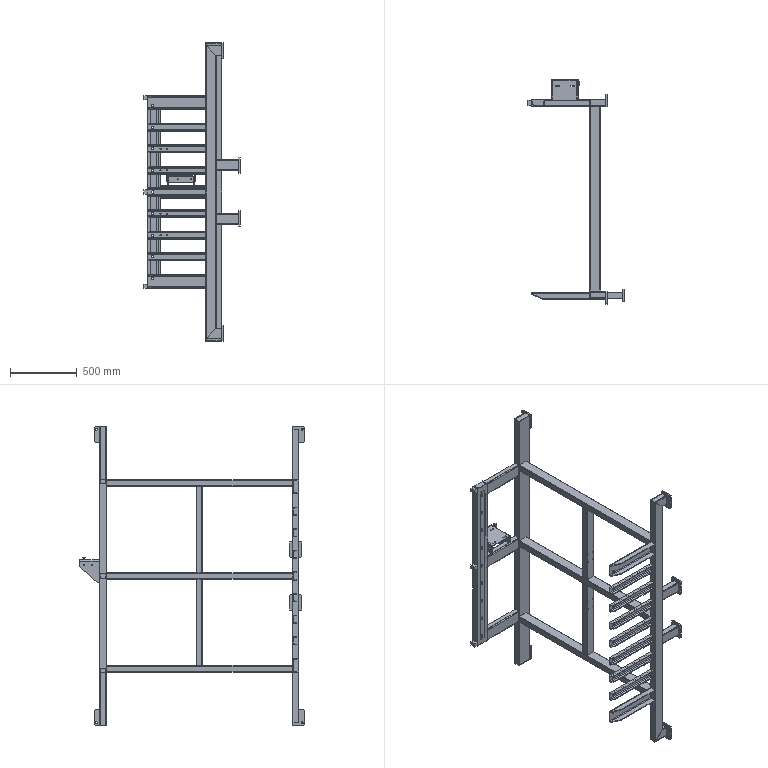Part | SolidWorks | features CompositeCurve 7 | 46 solids | 756 faces | box 720.5 x 1683 x 2240 mm | volume 17379745 mm3 | plane 461 | cylinder 295 | commonest cylinder face diameters 10 x48 17 x38 6 x32 2 x28 4 x28 8 x26